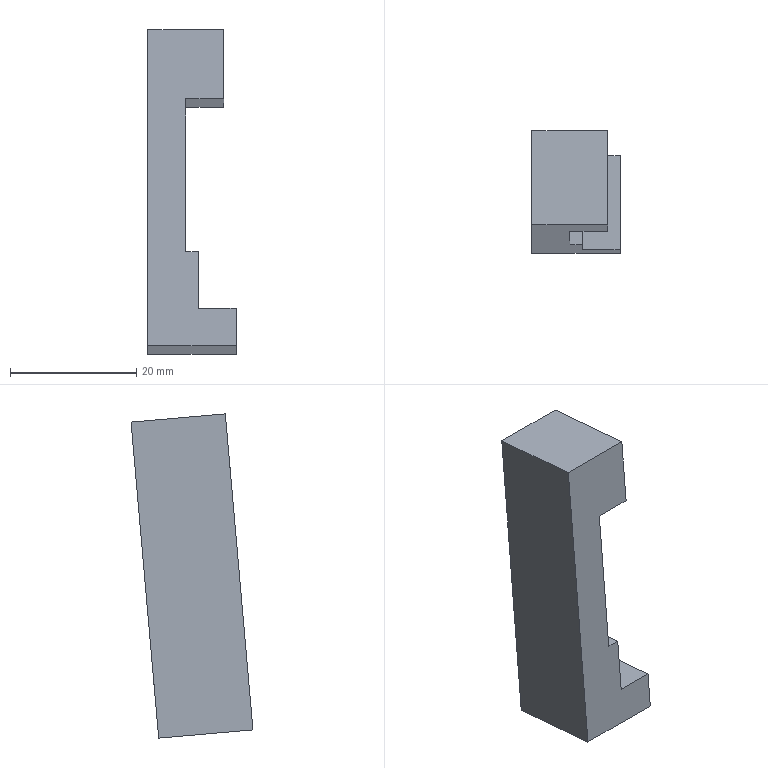Part | NX | features solid 2 | 1 solid | 12 faces | box 14 x 19.33 x 51.45 mm | volume 6510 mm3 | plane 12
STEP:
#1=CARTESIAN_POINT('',(87.,-189.065,-71.947));
#2=VERTEX_POINT('',#1);
#3=CARTESIAN_POINT('',(87.,-191.186,-96.188));
#4=VERTEX_POINT('',#3);
#5=CARTESIAN_POINT('',(87.,-188.106,-60.988));
#6=DIRECTION('',(0.,-0.08716,-0.9962));
#7=VECTOR('',#6,1000.);
#8=LINE('',#5,#7);
#9=EDGE_CURVE('',#2,#4,#8,.T.);
#10=ORIENTED_EDGE('',*,*,#9,.F.);
#11=CARTESIAN_POINT('',(87.,-204.008,-70.639));
#12=VERTEX_POINT('',#11);
#13=CARTESIAN_POINT('',(87.,-189.065,-71.947));
#14=DIRECTION('',(0.,0.9962,-0.08716));
#15=VECTOR('',#14,1000.);
#16=LINE('',#13,#15);
#17=EDGE_CURVE('',#2,#12,#16,.F.);
#18=ORIENTED_EDGE('',*,*,#17,.T.);
#19=CARTESIAN_POINT('',(87.,-206.129,-94.881));
#20=VERTEX_POINT('',#19);
#21=CARTESIAN_POINT('',(87.,-203.049,-59.681));
#22=DIRECTION('',(0.,-0.08716,-0.9962));
#23=VECTOR('',#22,1000.);
#24=LINE('',#21,#23);
#25=EDGE_CURVE('',#12,#20,#24,.T.);
#26=ORIENTED_EDGE('',*,*,#25,.T.);
#27=CARTESIAN_POINT('',(87.,-191.186,-96.188));
#28=DIRECTION('',(0.,0.9962,-0.08716));
#29=VECTOR('',#28,1000.);
#30=LINE('',#27,#29);
#31=EDGE_CURVE('',#4,#20,#30,.F.);
#32=ORIENTED_EDGE('',*,*,#31,.F.);
#33=EDGE_LOOP('',(#10,#18,#26,#32));
#34=FACE_BOUND('',#33,.T.);
#35=CARTESIAN_POINT('',(87.,-217.992,-58.374));
#36=DIRECTION('',(-1.,0.,0.));
#37=DIRECTION('',(0.,-0.08716,-0.9962));
#38=AXIS2_PLACEMENT_3D('',#35,#36,#37);
#39=PLANE('',#38);
#40=ADVANCED_FACE('',(#34),#39,.F.);
#41=CARTESIAN_POINT('',(81.,-188.106,-60.988));
#42=VERTEX_POINT('',#41);
#43=CARTESIAN_POINT('',(81.,-203.049,-59.681));
#44=VERTEX_POINT('',#43);
#45=CARTESIAN_POINT('',(81.,-217.992,-58.374));
#46=DIRECTION('',(0.,0.9962,-0.08716));
#47=VECTOR('',#46,1000.);
#48=LINE('',#45,#47);
#49=EDGE_CURVE('',#42,#44,#48,.F.);
#50=ORIENTED_EDGE('',*,*,#49,.F.);
#51=CARTESIAN_POINT('',(81.,-192.493,-111.131));
#52=VERTEX_POINT('',#51);
#53=CARTESIAN_POINT('',(81.,-188.106,-60.988));
#54=DIRECTION('',(0.,-0.08716,-0.9962));
#55=VECTOR('',#54,1000.);
#56=LINE('',#53,#55);
#57=EDGE_CURVE('',#42,#52,#56,.T.);
#58=ORIENTED_EDGE('',*,*,#57,.T.);
#59=CARTESIAN_POINT('',(81.,-207.436,-109.824));
#60=VERTEX_POINT('',#59);
#61=CARTESIAN_POINT('',(81.,-222.379,-108.517));
#62=DIRECTION('',(0.,-0.9962,0.08716));
#63=VECTOR('',#62,1000.);
#64=LINE('',#61,#63);
#65=EDGE_CURVE('',#52,#60,#64,.T.);
#66=ORIENTED_EDGE('',*,*,#65,.T.);
#67=CARTESIAN_POINT('',(81.,-203.049,-59.681));
#68=DIRECTION('',(0.,-0.08716,-0.9962));
#69=VECTOR('',#68,1000.);
#70=LINE('',#67,#69);
#71=EDGE_CURVE('',#44,#60,#70,.T.);
#72=ORIENTED_EDGE('',*,*,#71,.F.);
#73=EDGE_LOOP('',(#50,#58,#66,#72));
#74=FACE_BOUND('',#73,.T.);
#75=CARTESIAN_POINT('',(81.,-217.992,-58.374));
#76=DIRECTION('',(-1.,0.,0.));
#77=DIRECTION('',(0.,-0.08716,-0.9962));
#78=AXIS2_PLACEMENT_3D('',#75,#76,#77);
#79=PLANE('',#78);
#80=ADVANCED_FACE('',(#74),#79,.T.);
#81=ORIENTED_EDGE('',*,*,#65,.F.);
#82=CARTESIAN_POINT('',(95.,-192.493,-111.131));
#83=VERTEX_POINT('',#82);
#84=CARTESIAN_POINT('',(81.,-192.493,-111.131));
#85=DIRECTION('',(-1.,0.,0.));
#86=VECTOR('',#85,1000.);
#87=LINE('',#84,#86);
#88=EDGE_CURVE('',#52,#83,#87,.F.);
#89=ORIENTED_EDGE('',*,*,#88,.T.);
#90=CARTESIAN_POINT('',(95.,-207.436,-109.824));
#91=VERTEX_POINT('',#90);
#92=CARTESIAN_POINT('',(95.,-192.493,-111.131));
#93=DIRECTION('',(0.,-0.9962,0.08716));
#94=VECTOR('',#93,1000.);
#95=LINE('',#92,#94);
#96=EDGE_CURVE('',#83,#91,#95,.T.);
#97=ORIENTED_EDGE('',*,*,#96,.T.);
#98=CARTESIAN_POINT('',(81.,-207.436,-109.824));
#99=DIRECTION('',(-1.,0.,0.));
#100=VECTOR('',#99,1000.);
#101=LINE('',#98,#100);
#102=EDGE_CURVE('',#60,#91,#101,.F.);
#103=ORIENTED_EDGE('',*,*,#102,.F.);
#104=EDGE_LOOP('',(#81,#89,#97,#103));
#105=FACE_BOUND('',#104,.T.);
#106=CARTESIAN_POINT('',(81.,-222.379,-108.517));
#107=DIRECTION('',(0.,-0.08716,-0.9962));
#108=DIRECTION('',(1.,0.,0.));
#109=AXIS2_PLACEMENT_3D('',#106,#107,#108);
#110=PLANE('',#109);
#111=ADVANCED_FACE('',(#105),#110,.T.);
#112=CARTESIAN_POINT('',(93.,-188.106,-60.988));
#113=VERTEX_POINT('',#112);
#114=CARTESIAN_POINT('',(81.,-188.106,-60.988));
#115=DIRECTION('',(1.,0.,0.));
#116=VECTOR('',#115,1000.);
#117=LINE('',#114,#116);
#118=EDGE_CURVE('',#42,#113,#117,.T.);
#119=ORIENTED_EDGE('',*,*,#118,.F.);
#120=ORIENTED_EDGE('',*,*,#49,.T.);
#121=CARTESIAN_POINT('',(93.,-203.049,-59.681));
#122=VERTEX_POINT('',#121);
#123=CARTESIAN_POINT('',(81.,-203.049,-59.681));
#124=DIRECTION('',(1.,0.,0.));
#125=VECTOR('',#124,1000.);
#126=LINE('',#123,#125);
#127=EDGE_CURVE('',#44,#122,#126,.T.);
#128=ORIENTED_EDGE('',*,*,#127,.T.);
#129=CARTESIAN_POINT('',(93.,-188.106,-60.988));
#130=DIRECTION('',(0.,-0.9962,0.08716));
#131=VECTOR('',#130,1000.);
#132=LINE('',#129,#131);
#133=EDGE_CURVE('',#113,#122,#132,.T.);
#134=ORIENTED_EDGE('',*,*,#133,.F.);
#135=EDGE_LOOP('',(#119,#120,#128,#134));
#136=FACE_BOUND('',#135,.T.);
#137=CARTESIAN_POINT('',(81.,-217.992,-58.374));
#138=DIRECTION('',(0.,-0.08716,-0.9962));
#139=DIRECTION('',(1.,0.,0.));
#140=AXIS2_PLACEMENT_3D('',#137,#138,#139);
#141=PLANE('',#140);
#142=ADVANCED_FACE('',(#136),#141,.F.);
#143=ORIENTED_EDGE('',*,*,#127,.F.);
#144=ORIENTED_EDGE('',*,*,#71,.T.);
#145=ORIENTED_EDGE('',*,*,#102,.T.);
#146=CARTESIAN_POINT('',(95.,-206.913,-103.847));
#147=VERTEX_POINT('',#146);
#148=CARTESIAN_POINT('',(95.,-207.436,-109.824));
#149=DIRECTION('',(0.,-0.08716,-0.9962));
#150=VECTOR('',#149,1000.);
#151=LINE('',#148,#150);
#152=EDGE_CURVE('',#91,#147,#151,.F.);
#153=ORIENTED_EDGE('',*,*,#152,.T.);
#154=CARTESIAN_POINT('',(89.,-206.913,-103.847));
#155=VERTEX_POINT('',#154);
#156=CARTESIAN_POINT('',(95.,-206.913,-103.847));
#157=DIRECTION('',(1.,0.,0.));
#158=VECTOR('',#157,1000.);
#159=LINE('',#156,#158);
#160=EDGE_CURVE('',#147,#155,#159,.F.);
#161=ORIENTED_EDGE('',*,*,#160,.T.);
#162=CARTESIAN_POINT('',(89.,-206.129,-94.881));
#163=VERTEX_POINT('',#162);
#164=CARTESIAN_POINT('',(89.,-207.436,-109.824));
#165=DIRECTION('',(0.,-0.08716,-0.9962));
#166=VECTOR('',#165,1000.);
#167=LINE('',#164,#166);
#168=EDGE_CURVE('',#155,#163,#167,.F.);
#169=ORIENTED_EDGE('',*,*,#168,.T.);
#170=CARTESIAN_POINT('',(89.,-206.129,-94.881));
#171=DIRECTION('',(1.,0.,0.));
#172=VECTOR('',#171,1000.);
#173=LINE('',#170,#172);
#174=EDGE_CURVE('',#163,#20,#173,.F.);
#175=ORIENTED_EDGE('',*,*,#174,.T.);
#176=ORIENTED_EDGE('',*,*,#25,.F.);
#177=CARTESIAN_POINT('',(93.,-204.008,-70.639));
#178=VERTEX_POINT('',#177);
#179=CARTESIAN_POINT('',(93.,-204.008,-70.639));
#180=DIRECTION('',(1.,0.,0.));
#181=VECTOR('',#180,1000.);
#182=LINE('',#179,#181);
#183=EDGE_CURVE('',#178,#12,#182,.F.);
#184=ORIENTED_EDGE('',*,*,#183,.F.);
#185=CARTESIAN_POINT('',(93.,-203.049,-59.681));
#186=DIRECTION('',(0.,0.08716,0.9962));
#187=VECTOR('',#186,1000.);
#188=LINE('',#185,#187);
#189=EDGE_CURVE('',#122,#178,#188,.F.);
#190=ORIENTED_EDGE('',*,*,#189,.F.);
#191=EDGE_LOOP('',(#143,#144,#145,#153,#161,#169,#175,#176,#184,#190));
#192=FACE_BOUND('',#191,.T.);
#193=CARTESIAN_POINT('',(81.,-203.049,-59.681));
#194=DIRECTION('',(0.,0.9962,-0.08716));
#195=DIRECTION('',(0.,-0.08716,-0.9962));
#196=AXIS2_PLACEMENT_3D('',#193,#194,#195);
#197=PLANE('',#196);
#198=ADVANCED_FACE('',(#192),#197,.F.);
#199=ORIENTED_EDGE('',*,*,#9,.T.);
#200=CARTESIAN_POINT('',(89.,-191.186,-96.188));
#201=VERTEX_POINT('',#200);
#202=CARTESIAN_POINT('',(89.,-191.186,-96.188));
#203=DIRECTION('',(1.,0.,0.));
#204=VECTOR('',#203,1000.);
#205=LINE('',#202,#204);
#206=EDGE_CURVE('',#201,#4,#205,.F.);
#207=ORIENTED_EDGE('',*,*,#206,.F.);
#208=CARTESIAN_POINT('',(89.,-191.97,-105.154));
#209=VERTEX_POINT('',#208);
#210=CARTESIAN_POINT('',(89.,-192.493,-111.131));
#211=DIRECTION('',(0.,-0.08716,-0.9962));
#212=VECTOR('',#211,1000.);
#213=LINE('',#210,#212);
#214=EDGE_CURVE('',#209,#201,#213,.F.);
#215=ORIENTED_EDGE('',*,*,#214,.F.);
#216=CARTESIAN_POINT('',(95.,-191.97,-105.154));
#217=VERTEX_POINT('',#216);
#218=CARTESIAN_POINT('',(95.,-191.97,-105.154));
#219=DIRECTION('',(1.,0.,0.));
#220=VECTOR('',#219,1000.);
#221=LINE('',#218,#220);
#222=EDGE_CURVE('',#217,#209,#221,.F.);
#223=ORIENTED_EDGE('',*,*,#222,.F.);
#224=CARTESIAN_POINT('',(95.,-192.493,-111.131));
#225=DIRECTION('',(0.,-0.08716,-0.9962));
#226=VECTOR('',#225,1000.);
#227=LINE('',#224,#226);
#228=EDGE_CURVE('',#83,#217,#227,.F.);
#229=ORIENTED_EDGE('',*,*,#228,.F.);
#230=ORIENTED_EDGE('',*,*,#88,.F.);
#231=ORIENTED_EDGE('',*,*,#57,.F.);
#232=ORIENTED_EDGE('',*,*,#118,.T.);
#233=CARTESIAN_POINT('',(93.,-189.065,-71.947));
#234=VERTEX_POINT('',#233);
#235=CARTESIAN_POINT('',(93.,-188.106,-60.988));
#236=DIRECTION('',(0.,0.08716,0.9962));
#237=VECTOR('',#236,1000.);
#238=LINE('',#235,#237);
#239=EDGE_CURVE('',#113,#234,#238,.F.);
#240=ORIENTED_EDGE('',*,*,#239,.T.);
#241=CARTESIAN_POINT('',(93.,-189.065,-71.947));
#242=DIRECTION('',(1.,0.,0.));
#243=VECTOR('',#242,1000.);
#244=LINE('',#241,#243);
#245=EDGE_CURVE('',#234,#2,#244,.F.);
#246=ORIENTED_EDGE('',*,*,#245,.T.);
#247=EDGE_LOOP('',(#199,#207,#215,#223,#229,#230,#231,#232,#240,#246));
#248=FACE_BOUND('',#247,.T.);
#249=CARTESIAN_POINT('',(81.,-188.106,-60.988));
#250=DIRECTION('',(0.,0.9962,-0.08716));
#251=DIRECTION('',(0.,-0.08716,-0.9962));
#252=AXIS2_PLACEMENT_3D('',#249,#250,#251);
#253=PLANE('',#252);
#254=ADVANCED_FACE('',(#248),#253,.T.);
#255=ORIENTED_EDGE('',*,*,#239,.F.);
#256=ORIENTED_EDGE('',*,*,#133,.T.);
#257=ORIENTED_EDGE('',*,*,#189,.T.);
#258=CARTESIAN_POINT('',(93.,-189.065,-71.947));
#259=DIRECTION('',(0.,0.9962,-0.08716));
#260=VECTOR('',#259,1000.);
#261=LINE('',#258,#260);
#262=EDGE_CURVE('',#234,#178,#261,.F.);
#263=ORIENTED_EDGE('',*,*,#262,.F.);
#264=EDGE_LOOP('',(#255,#256,#257,#263));
#265=FACE_BOUND('',#264,.T.);
#266=CARTESIAN_POINT('',(93.,-188.106,-60.988));
#267=DIRECTION('',(1.,0.,0.));
#268=DIRECTION('',(0.,-0.9962,0.08716));
#269=AXIS2_PLACEMENT_3D('',#266,#267,#268);
#270=PLANE('',#269);
#271=ADVANCED_FACE('',(#265),#270,.T.);
#272=ORIENTED_EDGE('',*,*,#17,.F.);
#273=ORIENTED_EDGE('',*,*,#245,.F.);
#274=ORIENTED_EDGE('',*,*,#262,.T.);
#275=ORIENTED_EDGE('',*,*,#183,.T.);
#276=EDGE_LOOP('',(#272,#273,#274,#275));
#277=FACE_BOUND('',#276,.T.);
#278=CARTESIAN_POINT('',(93.,-189.065,-71.947));
#279=DIRECTION('',(0.,0.08716,0.9962));
#280=DIRECTION('',(0.,0.9962,-0.08716));
#281=AXIS2_PLACEMENT_3D('',#278,#279,#280);
#282=PLANE('',#281);
#283=ADVANCED_FACE('',(#277),#282,.F.);
#284=ORIENTED_EDGE('',*,*,#214,.T.);
#285=CARTESIAN_POINT('',(89.,-191.186,-96.188));
#286=DIRECTION('',(0.,0.9962,-0.08716));
#287=VECTOR('',#286,1000.);
#288=LINE('',#285,#287);
#289=EDGE_CURVE('',#201,#163,#288,.F.);
#290=ORIENTED_EDGE('',*,*,#289,.T.);
#291=ORIENTED_EDGE('',*,*,#168,.F.);
#292=CARTESIAN_POINT('',(89.,-191.97,-105.154));
#293=DIRECTION('',(0.,0.9962,-0.08716));
#294=VECTOR('',#293,1000.);
#295=LINE('',#292,#294);
#296=EDGE_CURVE('',#209,#155,#295,.F.);
#297=ORIENTED_EDGE('',*,*,#296,.F.);
#298=EDGE_LOOP('',(#284,#290,#291,#297));
#299=FACE_BOUND('',#298,.T.);
#300=CARTESIAN_POINT('',(89.,-192.493,-111.131));
#301=DIRECTION('',(1.,0.,0.));
#302=DIRECTION('',(0.,-0.9962,0.08716));
#303=AXIS2_PLACEMENT_3D('',#300,#301,#302);
#304=PLANE('',#303);
#305=ADVANCED_FACE('',(#299),#304,.T.);
#306=ORIENTED_EDGE('',*,*,#31,.T.);
#307=ORIENTED_EDGE('',*,*,#174,.F.);
#308=ORIENTED_EDGE('',*,*,#289,.F.);
#309=ORIENTED_EDGE('',*,*,#206,.T.);
#310=EDGE_LOOP('',(#306,#307,#308,#309));
#311=FACE_BOUND('',#310,.T.);
#312=CARTESIAN_POINT('',(89.,-191.186,-96.188));
#313=DIRECTION('',(0.,0.08716,0.9962));
#314=DIRECTION('',(0.,0.9962,-0.08716));
#315=AXIS2_PLACEMENT_3D('',#312,#313,#314);
#316=PLANE('',#315);
#317=ADVANCED_FACE('',(#311),#316,.T.);
#318=ORIENTED_EDGE('',*,*,#152,.F.);
#319=ORIENTED_EDGE('',*,*,#96,.F.);
#320=ORIENTED_EDGE('',*,*,#228,.T.);
#321=CARTESIAN_POINT('',(95.,-191.97,-105.154));
#322=DIRECTION('',(0.,0.9962,-0.08716));
#323=VECTOR('',#322,1000.);
#324=LINE('',#321,#323);
#325=EDGE_CURVE('',#217,#147,#324,.F.);
#326=ORIENTED_EDGE('',*,*,#325,.T.);
#327=EDGE_LOOP('',(#318,#319,#320,#326));
#328=FACE_BOUND('',#327,.T.);
#329=CARTESIAN_POINT('',(95.,-192.493,-111.131));
#330=DIRECTION('',(1.,0.,0.));
#331=DIRECTION('',(0.,-0.9962,0.08716));
#332=AXIS2_PLACEMENT_3D('',#329,#330,#331);
#333=PLANE('',#332);
#334=ADVANCED_FACE('',(#328),#333,.T.);
#335=ORIENTED_EDGE('',*,*,#296,.T.);
#336=ORIENTED_EDGE('',*,*,#160,.F.);
#337=ORIENTED_EDGE('',*,*,#325,.F.);
#338=ORIENTED_EDGE('',*,*,#222,.T.);
#339=EDGE_LOOP('',(#335,#336,#337,#338));
#340=FACE_BOUND('',#339,.T.);
#341=CARTESIAN_POINT('',(95.,-191.97,-105.154));
#342=DIRECTION('',(0.,0.08716,0.9962));
#343=DIRECTION('',(0.,0.9962,-0.08716));
#344=AXIS2_PLACEMENT_3D('',#341,#342,#343);
#345=PLANE('',#344);
#346=ADVANCED_FACE('',(#340),#345,.T.);
#347=CLOSED_SHELL('',(#40,#80,#111,#142,#198,#254,#271,#283,#305,#317,#334,#346));
#348=MANIFOLD_SOLID_BREP('',#347);
#349=(LENGTH_UNIT()NAMED_UNIT(*)SI_UNIT(.MILLI.,.METRE.));
#350=UNCERTAINTY_MEASURE_WITH_UNIT(LENGTH_MEASURE(0.00001),#349,'','');
#351=(NAMED_UNIT(*)PLANE_ANGLE_UNIT()SI_UNIT($,.RADIAN.));
#352=(NAMED_UNIT(*)SI_UNIT($,.STERADIAN.)SOLID_ANGLE_UNIT());
#353=(GEOMETRIC_REPRESENTATION_CONTEXT(3)GLOBAL_UNCERTAINTY_ASSIGNED_CONTEXT((#350))GLOBAL_UNIT_ASSIGNED_CONTEXT((#349,#351,#352))REPRESENTATION_CONTEXT('',''));
#354=ADVANCED_BREP_SHAPE_REPRESENTATION('',(#348),#353);